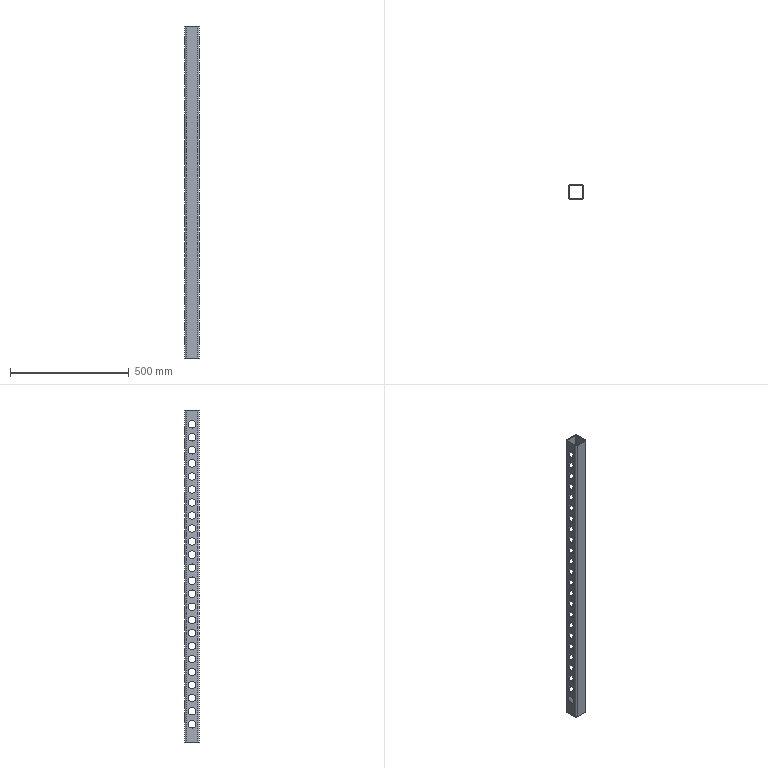Part | SolidWorks | features BaseBody 1 | 1 solid | 160 faces | box 60 x 60 x 1400 mm | volume 753847 mm3 | cylinder 150 | plane 10 | commonest cylinder face diameters 32 x142 6 x4 12 x4